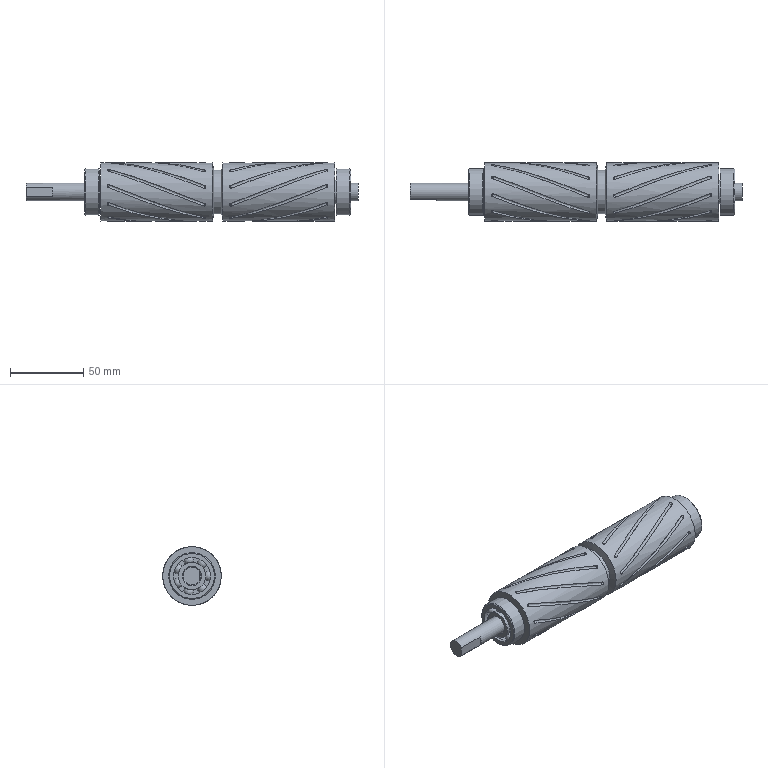Part | STEP file | YBQDJ-SSJ-7 | 1 solid | 187 faces | box 227 x 40.957 x 41.285 mm | volume 212732 mm3 | spline 60 | plane 56 | torus 28 | cylinder 17 | sphere 14 | cone 12 | commonest cylinder face diameters 12 x4 18.667 x4 25.333 x2 32 x2 40 x2 16 x1